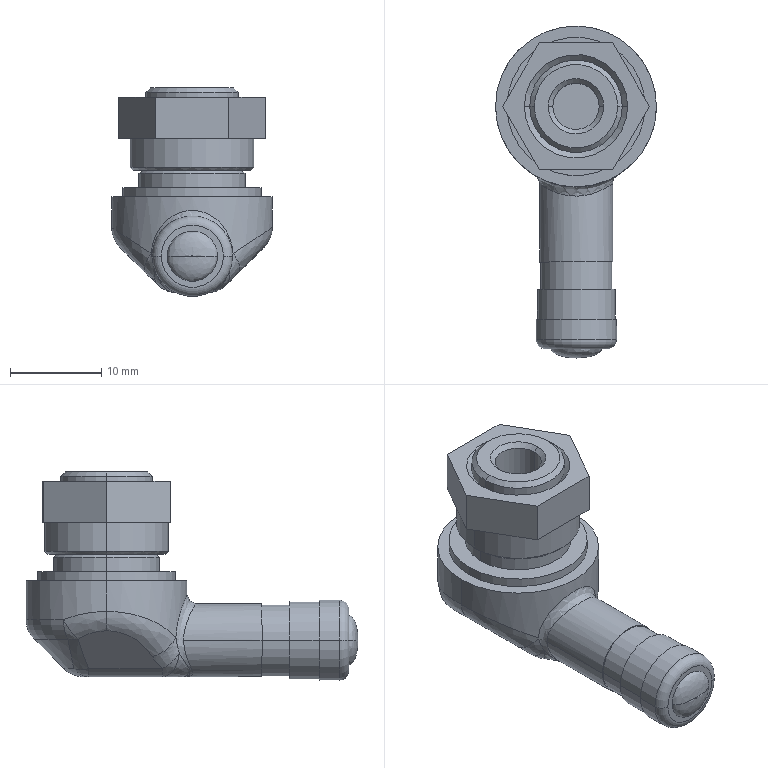Part | SolidWorks | features BaseBody 1 | 1 solid | 90 faces | box 17.6 x 36.3 x 22.8 mm | volume 4379 mm3 | cylinder 24 | plane 22 | spline 20 | cone 13 | sphere 7 | torus 4 | commonest cylinder face diameters 10.12 x4 5.065 x2 6 x2 7.8 x2 8 x2 8.5 x2